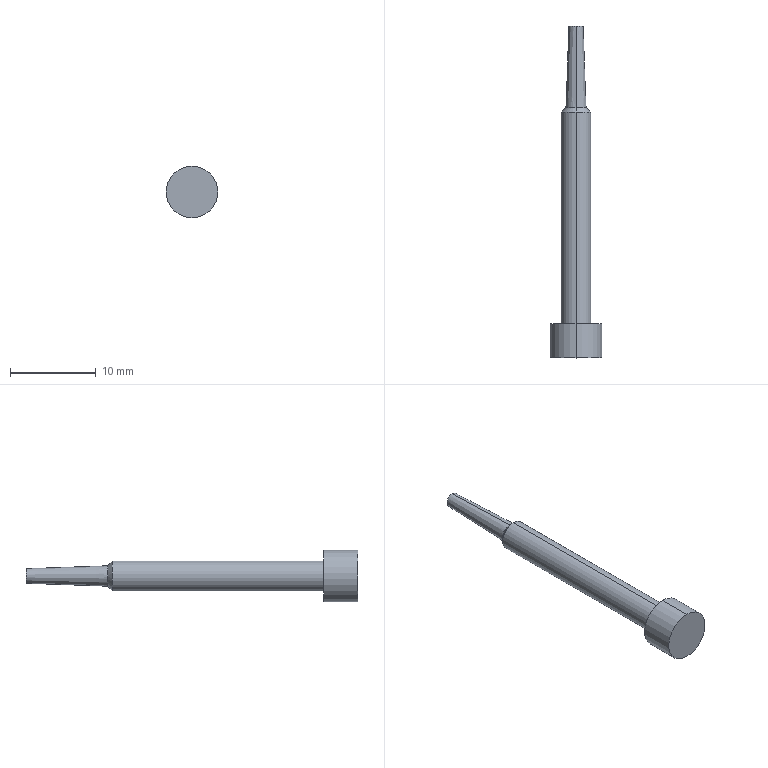Part | STEP file | 1 solid | 12 faces | box 6 x 38.743 x 6 mm | volume 385.655 mm3 | cylinder 4 | cone 4 | plane 4 | commonest cylinder face diameters 3.5 x2 6 x2
STEP:
#1=CARTESIAN_POINT('',(0.,0.,0.));
#2=DIRECTION('',(0.,0.,1.));
#3=DIRECTION('',(1.,0.,0.));
#4=AXIS2_PLACEMENT_3D('',#1,#2,#3);
#5=CARTESIAN_POINT('',(-137.183,-30.,14.557));
#6=VERTEX_POINT('',#5);
#7=CARTESIAN_POINT('',(-137.183,-30.,8.557));
#8=VERTEX_POINT('',#7);
#9=CARTESIAN_POINT('',(-137.183,-30.,11.557));
#10=DIRECTION('',(0.,1.,0.));
#11=DIRECTION('',(0.,0.,1.));
#12=AXIS2_PLACEMENT_3D('',#9,#10,#11);
#13=CIRCLE('',#12,3.);
#14=CARTESIAN_POINT('',(-137.183,-30.,11.557));
#15=DIRECTION('',(0.,1.,0.));
#16=DIRECTION('',(0.,0.,1.));
#17=AXIS2_PLACEMENT_3D('',#14,#15,#16);
#18=CYLINDRICAL_SURFACE('',#17,3.);
#19=CARTESIAN_POINT('',(0.,0.));
#20=DIRECTION('',(1.,0.));
#21=VECTOR('',#20,1.);
#22=LINE('',#19,#21);
#23=(GEOMETRIC_REPRESENTATION_CONTEXT(2)PARAMETRIC_REPRESENTATION_CONTEXT()REPRESENTATION_CONTEXT('',''));
#24=DEFINITIONAL_REPRESENTATION('',(#22),#23);
#25=PCURVE('',#18,#24);
#26=CARTESIAN_POINT('',(-72.862,-30.,115.03));
#27=DIRECTION('',(0.,1.,0.));
#28=DIRECTION('',(0.,0.,1.));
#29=AXIS2_PLACEMENT_3D('',#26,#27,#28);
#30=PLANE('',#29);
#31=CARTESIAN_POINT('',(-103.472,-64.32));
#32=DIRECTION('',(1.,0.));
#33=AXIS2_PLACEMENT_2D('',#31,#32);
#34=CIRCLE('',#33,3.);
#35=(GEOMETRIC_REPRESENTATION_CONTEXT(2)PARAMETRIC_REPRESENTATION_CONTEXT()REPRESENTATION_CONTEXT('',''));
#36=DEFINITIONAL_REPRESENTATION('',(#34),#35);
#37=PCURVE('',#30,#36);
#38=SURFACE_CURVE('',#13,(#25,#37),.PCURVE_S1.);
#39=EDGE_CURVE('',#6,#8,#38,.T.);
#40=ORIENTED_EDGE('',*,*,#39,.T.);
#41=CARTESIAN_POINT('',(-137.183,-26.,8.557));
#42=VERTEX_POINT('',#41);
#43=CARTESIAN_POINT('',(-137.183,-30.,8.557));
#44=DIRECTION('',(0.,1.,0.));
#45=VECTOR('',#44,1.);
#46=LINE('',#43,#45);
#47=CARTESIAN_POINT('',(3.142,0.));
#48=DIRECTION('',(0.,1.));
#49=VECTOR('',#48,1.);
#50=LINE('',#47,#49);
#51=(GEOMETRIC_REPRESENTATION_CONTEXT(2)PARAMETRIC_REPRESENTATION_CONTEXT()REPRESENTATION_CONTEXT('',''));
#52=DEFINITIONAL_REPRESENTATION('',(#50),#51);
#53=PCURVE('',#18,#52);
#54=CARTESIAN_POINT('',(-137.183,-30.,11.557));
#55=DIRECTION('',(0.,1.,0.));
#56=DIRECTION('',(0.,0.,1.));
#57=AXIS2_PLACEMENT_3D('',#54,#55,#56);
#58=CYLINDRICAL_SURFACE('',#57,3.);
#59=CARTESIAN_POINT('',(3.142,0.));
#60=DIRECTION('',(0.,1.));
#61=VECTOR('',#60,1.);
#62=LINE('',#59,#61);
#63=(GEOMETRIC_REPRESENTATION_CONTEXT(2)PARAMETRIC_REPRESENTATION_CONTEXT()REPRESENTATION_CONTEXT('',''));
#64=DEFINITIONAL_REPRESENTATION('',(#62),#63);
#65=PCURVE('',#58,#64);
#66=SURFACE_CURVE('',#46,(#53,#65),.PCURVE_S1.);
#67=EDGE_CURVE('',#8,#42,#66,.T.);
#68=ORIENTED_EDGE('',*,*,#67,.T.);
#69=CARTESIAN_POINT('',(-137.183,-26.,14.557));
#70=VERTEX_POINT('',#69);
#71=CARTESIAN_POINT('',(-137.183,-26.,11.557));
#72=DIRECTION('',(0.,-1.,0.));
#73=DIRECTION('',(0.,0.,-1.));
#74=AXIS2_PLACEMENT_3D('',#71,#72,#73);
#75=CIRCLE('',#74,3.);
#76=CARTESIAN_POINT('',(3.142,4.));
#77=DIRECTION('',(-1.,0.));
#78=VECTOR('',#77,1.);
#79=LINE('',#76,#78);
#80=(GEOMETRIC_REPRESENTATION_CONTEXT(2)PARAMETRIC_REPRESENTATION_CONTEXT()REPRESENTATION_CONTEXT('',''));
#81=DEFINITIONAL_REPRESENTATION('',(#79),#80);
#82=PCURVE('',#18,#81);
#83=CARTESIAN_POINT('',(-137.183,-26.,11.557));
#84=DIRECTION('',(0.,1.,0.));
#85=DIRECTION('',(0.,0.,1.));
#86=AXIS2_PLACEMENT_3D('',#83,#84,#85);
#87=PLANE('',#86);
#88=CARTESIAN_POINT('',(-3.,0.));
#89=CARTESIAN_POINT('',(-3.,5.196));
#90=CARTESIAN_POINT('',(1.5,2.598));
#91=CARTESIAN_POINT('',(6.,0.));
#92=CARTESIAN_POINT('',(1.5,-2.598));
#93=CARTESIAN_POINT('',(-3.,-5.196));
#94=CARTESIAN_POINT('',(-3.,0.));
#95=(BOUNDED_CURVE()B_SPLINE_CURVE(2,(#88,#89,#90,#91,#92,#93,#94),.UNSPECIFIED.,.T.,.F.)B_SPLINE_CURVE_WITH_KNOTS((1,2,2,2,2,1),(-2.094,0.,2.094,4.189,6.283,8.378),.UNSPECIFIED.)CURVE()GEOMETRIC_REPRESENTATION_ITEM()RATIONAL_B_SPLINE_CURVE((1.,0.5,1.,0.5,1.,0.5,1.))REPRESENTATION_ITEM(''));
#96=(GEOMETRIC_REPRESENTATION_CONTEXT(2)PARAMETRIC_REPRESENTATION_CONTEXT()REPRESENTATION_CONTEXT('',''));
#97=DEFINITIONAL_REPRESENTATION('',(#95),#96);
#98=PCURVE('',#87,#97);
#99=SURFACE_CURVE('',#75,(#82,#98),.PCURVE_S1.);
#100=EDGE_CURVE('',#42,#70,#99,.T.);
#101=ORIENTED_EDGE('',*,*,#100,.T.);
#102=CARTESIAN_POINT('',(-137.183,-30.,14.557));
#103=DIRECTION('',(0.,1.,0.));
#104=VECTOR('',#103,1.);
#105=LINE('',#102,#104);
#106=CARTESIAN_POINT('',(0.,0.));
#107=DIRECTION('',(0.,1.));
#108=VECTOR('',#107,1.);
#109=LINE('',#106,#108);
#110=(GEOMETRIC_REPRESENTATION_CONTEXT(2)PARAMETRIC_REPRESENTATION_CONTEXT()REPRESENTATION_CONTEXT('',''));
#111=DEFINITIONAL_REPRESENTATION('',(#109),#110);
#112=PCURVE('',#18,#111);
#113=CARTESIAN_POINT('',(6.283,0.));
#114=DIRECTION('',(0.,1.));
#115=VECTOR('',#114,1.);
#116=LINE('',#113,#115);
#117=(GEOMETRIC_REPRESENTATION_CONTEXT(2)PARAMETRIC_REPRESENTATION_CONTEXT()REPRESENTATION_CONTEXT('',''));
#118=DEFINITIONAL_REPRESENTATION('',(#116),#117);
#119=PCURVE('',#58,#118);
#120=SURFACE_CURVE('',#105,(#112,#119),.PCURVE_S1.);
#121=EDGE_CURVE('',#6,#70,#120,.T.);
#122=ORIENTED_EDGE('',*,*,#121,.F.);
#123=EDGE_LOOP('',(#40,#68,#101,#122));
#124=FACE_BOUND('',#123,.T.);
#125=ADVANCED_FACE('',(#124),#18,.T.);
#126=CARTESIAN_POINT('',(-137.183,-0.7858,10.37));
#127=VERTEX_POINT('',#126);
#128=CARTESIAN_POINT('',(-137.183,-0.7858,12.745));
#129=VERTEX_POINT('',#128);
#130=CARTESIAN_POINT('',(-137.183,-0.7858,11.557));
#131=DIRECTION('',(0.,-1.,0.));
#132=DIRECTION('',(0.,0.,1.));
#133=AXIS2_PLACEMENT_3D('',#130,#131,#132);
#134=CIRCLE('',#133,1.188);
#135=CARTESIAN_POINT('',(-137.183,-1.306,11.557));
#136=DIRECTION('',(0.,-1.,0.));
#137=DIRECTION('',(0.,0.,-1.));
#138=AXIS2_PLACEMENT_3D('',#135,#136,#137);
#139=CONICAL_SURFACE('',#138,1.708,0.7854);
#140=CARTESIAN_POINT('',(-3.142,-0.5207));
#141=DIRECTION('',(1.,0.));
#142=VECTOR('',#141,1.);
#143=LINE('',#140,#142);
#144=(GEOMETRIC_REPRESENTATION_CONTEXT(2)PARAMETRIC_REPRESENTATION_CONTEXT()REPRESENTATION_CONTEXT('',''));
#145=DEFINITIONAL_REPRESENTATION('',(#143),#144);
#146=PCURVE('',#139,#145);
#147=CARTESIAN_POINT('',(-137.183,-1.306,11.557));
#148=DIRECTION('',(0.,-1.,0.));
#149=DIRECTION('',(0.,0.,-1.));
#150=AXIS2_PLACEMENT_3D('',#147,#148,#149);
#151=CONICAL_SURFACE('',#150,1.206,0.03491);
#152=CARTESIAN_POINT('',(-3.142,-0.5207));
#153=DIRECTION('',(1.,0.));
#154=VECTOR('',#153,1.);
#155=LINE('',#152,#154);
#156=(GEOMETRIC_REPRESENTATION_CONTEXT(2)PARAMETRIC_REPRESENTATION_CONTEXT()REPRESENTATION_CONTEXT('',''));
#157=DEFINITIONAL_REPRESENTATION('',(#155),#156);
#158=PCURVE('',#151,#157);
#159=SURFACE_CURVE('',#134,(#146,#158),.PCURVE_S1.);
#160=EDGE_CURVE('',#127,#129,#159,.T.);
#161=ORIENTED_EDGE('',*,*,#160,.T.);
#162=CARTESIAN_POINT('',(-137.183,-1.306,13.266));
#163=VERTEX_POINT('',#162);
#164=CARTESIAN_POINT('',(-137.183,-1.306,13.266));
#165=DIRECTION('',(0.,-0.7071,0.7071));
#166=VECTOR('',#165,1.);
#167=LINE('',#164,#166);
#168=CARTESIAN_POINT('',(3.142,0.));
#169=DIRECTION('',(0.,1.));
#170=VECTOR('',#169,1.);
#171=LINE('',#168,#170);
#172=(GEOMETRIC_REPRESENTATION_CONTEXT(2)PARAMETRIC_REPRESENTATION_CONTEXT()REPRESENTATION_CONTEXT('',''));
#173=DEFINITIONAL_REPRESENTATION('',(#171),#172);
#174=PCURVE('',#139,#173);
#175=CARTESIAN_POINT('',(-137.183,-1.306,11.557));
#176=DIRECTION('',(0.,-1.,0.));
#177=DIRECTION('',(0.,0.,-1.));
#178=AXIS2_PLACEMENT_3D('',#175,#176,#177);
#179=CONICAL_SURFACE('',#178,1.708,0.7854);
#180=CARTESIAN_POINT('',(3.142,0.));
#181=DIRECTION('',(0.,1.));
#182=VECTOR('',#181,1.);
#183=LINE('',#180,#182);
#184=(GEOMETRIC_REPRESENTATION_CONTEXT(2)PARAMETRIC_REPRESENTATION_CONTEXT()REPRESENTATION_CONTEXT('',''));
#185=DEFINITIONAL_REPRESENTATION('',(#183),#184);
#186=PCURVE('',#179,#185);
#187=SURFACE_CURVE('',#167,(#174,#186),.PCURVE_S1.);
#188=EDGE_CURVE('',#129,#163,#187,.T.);
#189=ORIENTED_EDGE('',*,*,#188,.T.);
#190=CARTESIAN_POINT('',(-137.183,-1.306,9.849));
#191=VERTEX_POINT('',#190);
#192=CARTESIAN_POINT('',(-137.183,-1.306,11.557));
#193=DIRECTION('',(0.,1.,0.));
#194=DIRECTION('',(0.,0.,-1.));
#195=AXIS2_PLACEMENT_3D('',#192,#193,#194);
#196=CIRCLE('',#195,1.708);
#197=CARTESIAN_POINT('',(6.283,0.));
#198=DIRECTION('',(-1.,0.));
#199=VECTOR('',#198,1.);
#200=LINE('',#197,#199);
#201=(GEOMETRIC_REPRESENTATION_CONTEXT(2)PARAMETRIC_REPRESENTATION_CONTEXT()REPRESENTATION_CONTEXT('',''));
#202=DEFINITIONAL_REPRESENTATION('',(#200),#201);
#203=PCURVE('',#139,#202);
#204=CARTESIAN_POINT('',(-137.183,-1.306,11.557));
#205=DIRECTION('',(0.,1.,0.));
#206=DIRECTION('',(0.,0.,1.));
#207=AXIS2_PLACEMENT_3D('',#204,#205,#206);
#208=PLANE('',#207);
#209=CARTESIAN_POINT('',(0.,0.));
#210=DIRECTION('',(-1.,0.));
#211=AXIS2_PLACEMENT_2D('',#209,#210);
#212=CIRCLE('',#211,1.708);
#213=(GEOMETRIC_REPRESENTATION_CONTEXT(2)PARAMETRIC_REPRESENTATION_CONTEXT()REPRESENTATION_CONTEXT('',''));
#214=DEFINITIONAL_REPRESENTATION('',(#212),#213);
#215=PCURVE('',#208,#214);
#216=SURFACE_CURVE('',#196,(#203,#215),.PCURVE_S1.);
#217=EDGE_CURVE('',#163,#191,#216,.T.);
#218=ORIENTED_EDGE('',*,*,#217,.T.);
#219=CARTESIAN_POINT('',(-137.183,-1.306,9.849));
#220=DIRECTION('',(0.,-0.7071,-0.7071));
#221=VECTOR('',#220,1.);
#222=LINE('',#219,#221);
#223=CARTESIAN_POINT('',(0.,0.));
#224=DIRECTION('',(0.,1.));
#225=VECTOR('',#224,1.);
#226=LINE('',#223,#225);
#227=(GEOMETRIC_REPRESENTATION_CONTEXT(2)PARAMETRIC_REPRESENTATION_CONTEXT()REPRESENTATION_CONTEXT('',''));
#228=DEFINITIONAL_REPRESENTATION('',(#226),#227);
#229=PCURVE('',#139,#228);
#230=CARTESIAN_POINT('',(6.283,0.));
#231=DIRECTION('',(0.,1.));
#232=VECTOR('',#231,1.);
#233=LINE('',#230,#232);
#234=(GEOMETRIC_REPRESENTATION_CONTEXT(2)PARAMETRIC_REPRESENTATION_CONTEXT()REPRESENTATION_CONTEXT('',''));
#235=DEFINITIONAL_REPRESENTATION('',(#233),#234);
#236=PCURVE('',#179,#235);
#237=SURFACE_CURVE('',#222,(#229,#236),.PCURVE_S1.);
#238=EDGE_CURVE('',#127,#191,#237,.T.);
#239=ORIENTED_EDGE('',*,*,#238,.F.);
#240=EDGE_LOOP('',(#161,#189,#218,#239));
#241=FACE_BOUND('',#240,.T.);
#242=ADVANCED_FACE('',(#241),#139,.T.);
#243=CARTESIAN_POINT('',(-137.183,8.743,10.702));
#244=VERTEX_POINT('',#243);
#245=CARTESIAN_POINT('',(-137.183,8.743,12.413));
#246=VERTEX_POINT('',#245);
#247=CARTESIAN_POINT('',(-137.183,8.743,11.557));
#248=DIRECTION('',(0.,-1.,0.));
#249=DIRECTION('',(0.,0.,-1.));
#250=AXIS2_PLACEMENT_3D('',#247,#248,#249);
#251=CIRCLE('',#250,0.855);
#252=CARTESIAN_POINT('',(0.,-10.05));
#253=DIRECTION('',(1.,0.));
#254=VECTOR('',#253,1.);
#255=LINE('',#252,#254);
#256=(GEOMETRIC_REPRESENTATION_CONTEXT(2)PARAMETRIC_REPRESENTATION_CONTEXT()REPRESENTATION_CONTEXT('',''));
#257=DEFINITIONAL_REPRESENTATION('',(#255),#256);
#258=PCURVE('',#151,#257);
#259=CARTESIAN_POINT('',(-137.183,8.743,9.849));
#260=DIRECTION('',(0.,1.,0.));
#261=DIRECTION('',(0.,0.,1.));
#262=AXIS2_PLACEMENT_3D('',#259,#260,#261);
#263=PLANE('',#262);
#264=CARTESIAN_POINT('',(0.8535,0.));
#265=CARTESIAN_POINT('',(0.8535,1.481));
#266=CARTESIAN_POINT('',(2.136,0.7405));
#267=CARTESIAN_POINT('',(3.419,0.));
#268=CARTESIAN_POINT('',(2.136,-0.7405));
#269=CARTESIAN_POINT('',(0.8535,-1.481));
#270=CARTESIAN_POINT('',(0.8535,0.));
#271=(BOUNDED_CURVE()B_SPLINE_CURVE(2,(#264,#265,#266,#267,#268,#269,#270),.UNSPECIFIED.,.T.,.F.)B_SPLINE_CURVE_WITH_KNOTS((1,2,2,2,2,1),(-2.094,0.,2.094,4.189,6.283,8.378),.UNSPECIFIED.)CURVE()GEOMETRIC_REPRESENTATION_ITEM()RATIONAL_B_SPLINE_CURVE((1.,0.5,1.,0.5,1.,0.5,1.))REPRESENTATION_ITEM(''));
#272=(GEOMETRIC_REPRESENTATION_CONTEXT(2)PARAMETRIC_REPRESENTATION_CONTEXT()REPRESENTATION_CONTEXT('',''));
#273=DEFINITIONAL_REPRESENTATION('',(#271),#272);
#274=PCURVE('',#263,#273);
#275=SURFACE_CURVE('',#251,(#258,#274),.PCURVE_S1.);
#276=EDGE_CURVE('',#244,#246,#275,.T.);
#277=ORIENTED_EDGE('',*,*,#276,.T.);
#278=CARTESIAN_POINT('',(-137.183,-1.306,12.764));
#279=DIRECTION('',(0.,-0.9994,0.0349));
#280=VECTOR('',#279,1.);
#281=LINE('',#278,#280);
#282=CARTESIAN_POINT('',(3.142,0.));
#283=DIRECTION('',(0.,1.));
#284=VECTOR('',#283,1.);
#285=LINE('',#282,#284);
#286=(GEOMETRIC_REPRESENTATION_CONTEXT(2)PARAMETRIC_REPRESENTATION_CONTEXT()REPRESENTATION_CONTEXT('',''));
#287=DEFINITIONAL_REPRESENTATION('',(#285),#286);
#288=PCURVE('',#151,#287);
#289=CARTESIAN_POINT('',(-137.183,-1.306,11.557));
#290=DIRECTION('',(0.,-1.,0.));
#291=DIRECTION('',(0.,0.,-1.));
#292=AXIS2_PLACEMENT_3D('',#289,#290,#291);
#293=CONICAL_SURFACE('',#292,1.206,0.03491);
#294=CARTESIAN_POINT('',(3.142,0.));
#295=DIRECTION('',(0.,1.));
#296=VECTOR('',#295,1.);
#297=LINE('',#294,#296);
#298=(GEOMETRIC_REPRESENTATION_CONTEXT(2)PARAMETRIC_REPRESENTATION_CONTEXT()REPRESENTATION_CONTEXT('',''));
#299=DEFINITIONAL_REPRESENTATION('',(#297),#298);
#300=PCURVE('',#293,#299);
#301=SURFACE_CURVE('',#281,(#288,#300),.PCURVE_S1.);
#302=EDGE_CURVE('',#246,#129,#301,.T.);
#303=ORIENTED_EDGE('',*,*,#302,.T.);
#304=ORIENTED_EDGE('',*,*,#160,.F.);
#305=CARTESIAN_POINT('',(-137.183,-1.306,10.351));
#306=DIRECTION('',(0.,-0.9994,-0.0349));
#307=VECTOR('',#306,1.);
#308=LINE('',#305,#307);
#309=CARTESIAN_POINT('',(0.,0.));
#310=DIRECTION('',(0.,1.));
#311=VECTOR('',#310,1.);
#312=LINE('',#309,#311);
#313=(GEOMETRIC_REPRESENTATION_CONTEXT(2)PARAMETRIC_REPRESENTATION_CONTEXT()REPRESENTATION_CONTEXT('',''));
#314=DEFINITIONAL_REPRESENTATION('',(#312),#313);
#315=PCURVE('',#151,#314);
#316=CARTESIAN_POINT('',(6.283,0.));
#317=DIRECTION('',(0.,1.));
#318=VECTOR('',#317,1.);
#319=LINE('',#316,#318);
#320=(GEOMETRIC_REPRESENTATION_CONTEXT(2)PARAMETRIC_REPRESENTATION_CONTEXT()REPRESENTATION_CONTEXT('',''));
#321=DEFINITIONAL_REPRESENTATION('',(#319),#320);
#322=PCURVE('',#293,#321);
#323=SURFACE_CURVE('',#308,(#315,#322),.PCURVE_S1.);
#324=EDGE_CURVE('',#244,#127,#323,.T.);
#325=ORIENTED_EDGE('',*,*,#324,.F.);
#326=EDGE_LOOP('',(#277,#303,#304,#325));
#327=FACE_BOUND('',#326,.T.);
#328=ADVANCED_FACE('',(#327),#151,.T.);
#329=CARTESIAN_POINT('',(-137.183,-1.306,9.807));
#330=VERTEX_POINT('',#329);
#331=CARTESIAN_POINT('',(-137.183,-1.306,13.307));
#332=VERTEX_POINT('',#331);
#333=CARTESIAN_POINT('',(-137.183,-1.306,11.557));
#334=DIRECTION('',(0.,-1.,0.));
#335=DIRECTION('',(0.,0.,-1.));
#336=AXIS2_PLACEMENT_3D('',#333,#334,#335);
#337=CIRCLE('',#336,1.75);
#338=CARTESIAN_POINT('',(-137.183,-1.306,11.557));
#339=DIRECTION('',(0.,-1.,0.));
#340=DIRECTION('',(0.,0.,-1.));
#341=AXIS2_PLACEMENT_3D('',#338,#339,#340);
#342=CYLINDRICAL_SURFACE('',#341,1.75);
#343=CARTESIAN_POINT('',(0.,0.));
#344=DIRECTION('',(1.,0.));
#345=VECTOR('',#344,1.);
#346=LINE('',#343,#345);
#347=(GEOMETRIC_REPRESENTATION_CONTEXT(2)PARAMETRIC_REPRESENTATION_CONTEXT()REPRESENTATION_CONTEXT('',''));
#348=DEFINITIONAL_REPRESENTATION('',(#346),#347);
#349=PCURVE('',#342,#348);
#350=CARTESIAN_POINT('',(-1.75,0.));
#351=CARTESIAN_POINT('',(-1.75,3.031));
#352=CARTESIAN_POINT('',(0.875,1.516));
#353=CARTESIAN_POINT('',(3.5,0.));
#354=CARTESIAN_POINT('',(0.875,-1.516));
#355=CARTESIAN_POINT('',(-1.75,-3.031));
#356=CARTESIAN_POINT('',(-1.75,0.));
#357=(BOUNDED_CURVE()B_SPLINE_CURVE(2,(#350,#351,#352,#353,#354,#355,#356),.UNSPECIFIED.,.T.,.F.)B_SPLINE_CURVE_WITH_KNOTS((1,2,2,2,2,1),(-2.094,0.,2.094,4.189,6.283,8.378),.UNSPECIFIED.)CURVE()GEOMETRIC_REPRESENTATION_ITEM()RATIONAL_B_SPLINE_CURVE((1.,0.5,1.,0.5,1.,0.5,1.))REPRESENTATION_ITEM(''));
#358=(GEOMETRIC_REPRESENTATION_CONTEXT(2)PARAMETRIC_REPRESENTATION_CONTEXT()REPRESENTATION_CONTEXT('',''));
#359=DEFINITIONAL_REPRESENTATION('',(#357),#358);
#360=PCURVE('',#208,#359);
#361=SURFACE_CURVE('',#337,(#349,#360),.PCURVE_S1.);
#362=EDGE_CURVE('',#330,#332,#361,.T.);
#363=ORIENTED_EDGE('',*,*,#362,.T.);
#364=CARTESIAN_POINT('',(-137.183,-26.,13.307));
#365=VERTEX_POINT('',#364);
#366=CARTESIAN_POINT('',(-137.183,-1.306,13.307));
#367=DIRECTION('',(0.,-1.,0.));
#368=VECTOR('',#367,1.);
#369=LINE('',#366,#368);
#370=CARTESIAN_POINT('',(3.142,0.));
#371=DIRECTION('',(0.,1.));
#372=VECTOR('',#371,1.);
#373=LINE('',#370,#372);
#374=(GEOMETRIC_REPRESENTATION_CONTEXT(2)PARAMETRIC_REPRESENTATION_CONTEXT()REPRESENTATION_CONTEXT('',''));
#375=DEFINITIONAL_REPRESENTATION('',(#373),#374);
#376=PCURVE('',#342,#375);
#377=CARTESIAN_POINT('',(-137.183,-1.306,11.557));
#378=DIRECTION('',(0.,-1.,0.));
#379=DIRECTION('',(0.,0.,-1.));
#380=AXIS2_PLACEMENT_3D('',#377,#378,#379);
#381=CYLINDRICAL_SURFACE('',#380,1.75);
#382=CARTESIAN_POINT('',(3.142,0.));
#383=DIRECTION('',(0.,1.));
#384=VECTOR('',#383,1.);
#385=LINE('',#382,#384);
#386=(GEOMETRIC_REPRESENTATION_CONTEXT(2)PARAMETRIC_REPRESENTATION_CONTEXT()REPRESENTATION_CONTEXT('',''));
#387=DEFINITIONAL_REPRESENTATION('',(#385),#386);
#388=PCURVE('',#381,#387);
#389=SURFACE_CURVE('',#369,(#376,#388),.PCURVE_S1.);
#390=EDGE_CURVE('',#332,#365,#389,.T.);
#391=ORIENTED_EDGE('',*,*,#390,.T.);
#392=CARTESIAN_POINT('',(-137.183,-26.,9.807));
#393=VERTEX_POINT('',#392);
#394=CARTESIAN_POINT('',(-137.183,-26.,11.557));
#395=DIRECTION('',(0.,-1.,0.));
#396=DIRECTION('',(0.,0.,1.));
#397=AXIS2_PLACEMENT_3D('',#394,#395,#396);
#398=CIRCLE('',#397,1.75);
#399=CARTESIAN_POINT('',(-3.142,24.694));
#400=DIRECTION('',(1.,0.));
#401=VECTOR('',#400,1.);
#402=LINE('',#399,#401);
#403=(GEOMETRIC_REPRESENTATION_CONTEXT(2)PARAMETRIC_REPRESENTATION_CONTEXT()REPRESENTATION_CONTEXT('',''));
#404=DEFINITIONAL_REPRESENTATION('',(#402),#403);
#405=PCURVE('',#342,#404);
#406=CARTESIAN_POINT('',(1.75,0.));
#407=CARTESIAN_POINT('',(1.75,-3.031));
#408=CARTESIAN_POINT('',(-0.875,-1.516));
#409=CARTESIAN_POINT('',(-3.5,0.));
#410=CARTESIAN_POINT('',(-0.875,1.516));
#411=CARTESIAN_POINT('',(1.75,3.031));
#412=CARTESIAN_POINT('',(1.75,0.));
#413=(BOUNDED_CURVE()B_SPLINE_CURVE(2,(#406,#407,#408,#409,#410,#411,#412),.UNSPECIFIED.,.T.,.F.)B_SPLINE_CURVE_WITH_KNOTS((1,2,2,2,2,1),(-2.094,0.,2.094,4.189,6.283,8.378),.UNSPECIFIED.)CURVE()GEOMETRIC_REPRESENTATION_ITEM()RATIONAL_B_SPLINE_CURVE((1.,0.5,1.,0.5,1.,0.5,1.))REPRESENTATION_ITEM(''));
#414=(GEOMETRIC_REPRESENTATION_CONTEXT(2)PARAMETRIC_REPRESENTATION_CONTEXT()REPRESENTATION_CONTEXT('',''));
#415=DEFINITIONAL_REPRESENTATION('',(#413),#414);
#416=PCURVE('',#87,#415);
#417=SURFACE_CURVE('',#398,(#405,#416),.PCURVE_S1.);
#418=EDGE_CURVE('',#393,#365,#417,.T.);
#419=ORIENTED_EDGE('',*,*,#418,.F.);
#420=CARTESIAN_POINT('',(-137.183,-1.306,9.807));
#421=DIRECTION('',(0.,-1.,0.));
#422=VECTOR('',#421,1.);
#423=LINE('',#420,#422);
#424=CARTESIAN_POINT('',(0.,0.));
#425=DIRECTION('',(0.,1.));
#426=VECTOR('',#425,1.);
#427=LINE('',#424,#426);
#428=(GEOMETRIC_REPRESENTATION_CONTEXT(2)PARAMETRIC_REPRESENTATION_CONTEXT()REPRESENTATION_CONTEXT('',''));
#429=DEFINITIONAL_REPRESENTATION('',(#427),#428);
#430=PCURVE('',#342,#429);
#431=CARTESIAN_POINT('',(6.283,0.));
#432=DIRECTION('',(0.,1.));
#433=VECTOR('',#432,1.);
#434=LINE('',#431,#433);
#435=(GEOMETRIC_REPRESENTATION_CONTEXT(2)PARAMETRIC_REPRESENTATION_CONTEXT()REPRESENTATION_CONTEXT('',''));
#436=DEFINITIONAL_REPRESENTATION('',(#434),#435);
#437=PCURVE('',#381,#436);
#438=SURFACE_CURVE('',#423,(#430,#437),.PCURVE_S1.);
#439=EDGE_CURVE('',#330,#393,#438,.T.);
#440=ORIENTED_EDGE('',*,*,#439,.F.);
#441=EDGE_LOOP('',(#363,#391,#419,#440));
#442=FACE_BOUND('',#441,.T.);
#443=ADVANCED_FACE('',(#442),#342,.T.);
#444=CARTESIAN_POINT('',(-137.183,-1.306,11.557));
#445=DIRECTION('',(0.,1.,0.));
#446=DIRECTION('',(0.,0.,-1.));
#447=AXIS2_PLACEMENT_3D('',#444,#445,#446);
#448=CIRCLE('',#447,1.708);
#449=CARTESIAN_POINT('',(0.,0.));
#450=DIRECTION('',(-1.,0.));
#451=AXIS2_PLACEMENT_2D('',#449,#450);
#452=CIRCLE('',#451,1.708);
#453=(GEOMETRIC_REPRESENTATION_CONTEXT(2)PARAMETRIC_REPRESENTATION_CONTEXT()REPRESENTATION_CONTEXT('',''));
#454=DEFINITIONAL_REPRESENTATION('',(#452),#453);
#455=PCURVE('',#208,#454);
#456=CARTESIAN_POINT('',(6.283,0.));
#457=DIRECTION('',(-1.,0.));
#458=VECTOR('',#457,1.);
#459=LINE('',#456,#458);
#460=(GEOMETRIC_REPRESENTATION_CONTEXT(2)PARAMETRIC_REPRESENTATION_CONTEXT()REPRESENTATION_CONTEXT('',''));
#461=DEFINITIONAL_REPRESENTATION('',(#459),#460);
#462=PCURVE('',#179,#461);
#463=SURFACE_CURVE('',#448,(#455,#462),.PCURVE_S1.);
#464=EDGE_CURVE('',#191,#163,#463,.T.);
#465=ORIENTED_EDGE('',*,*,#464,.F.);
#466=ORIENTED_EDGE('',*,*,#217,.F.);
#467=EDGE_LOOP('',(#465,#466));
#468=FACE_BOUND('',#467,.T.);
#469=ORIENTED_EDGE('',*,*,#362,.F.);
#470=CARTESIAN_POINT('',(-137.183,-1.306,11.557));
#471=DIRECTION('',(0.,-1.,0.));
#472=DIRECTION('',(0.,0.,-1.));
#473=AXIS2_PLACEMENT_3D('',#470,#471,#472);
#474=CIRCLE('',#473,1.75);
#475=CARTESIAN_POINT('',(-1.75,0.));
#476=CARTESIAN_POINT('',(-1.75,3.031));
#477=CARTESIAN_POINT('',(0.875,1.516));
#478=CARTESIAN_POINT('',(3.5,0.));
#479=CARTESIAN_POINT('',(0.875,-1.516));
#480=CARTESIAN_POINT('',(-1.75,-3.031));
#481=CARTESIAN_POINT('',(-1.75,0.));
#482=(BOUNDED_CURVE()B_SPLINE_CURVE(2,(#475,#476,#477,#478,#479,#480,#481),.UNSPECIFIED.,.T.,.F.)B_SPLINE_CURVE_WITH_KNOTS((1,2,2,2,2,1),(-2.094,0.,2.094,4.189,6.283,8.378),.UNSPECIFIED.)CURVE()GEOMETRIC_REPRESENTATION_ITEM()RATIONAL_B_SPLINE_CURVE((1.,0.5,1.,0.5,1.,0.5,1.))REPRESENTATION_ITEM(''));
#483=(GEOMETRIC_REPRESENTATION_CONTEXT(2)PARAMETRIC_REPRESENTATION_CONTEXT()REPRESENTATION_CONTEXT('',''));
#484=DEFINITIONAL_REPRESENTATION('',(#482),#483);
#485=PCURVE('',#208,#484);
#486=CARTESIAN_POINT('',(0.,0.));
#487=DIRECTION('',(1.,0.));
#488=VECTOR('',#487,1.);
#489=LINE('',#486,#488);
#490=(GEOMETRIC_REPRESENTATION_CONTEXT(2)PARAMETRIC_REPRESENTATION_CONTEXT()REPRESENTATION_CONTEXT('',''));
#491=DEFINITIONAL_REPRESENTATION('',(#489),#490);
#492=PCURVE('',#381,#491);
#493=SURFACE_CURVE('',#474,(#485,#492),.PCURVE_S1.);
#494=EDGE_CURVE('',#332,#330,#493,.T.);
#495=ORIENTED_EDGE('',*,*,#494,.F.);
#496=EDGE_LOOP('',(#469,#495));
#497=FACE_BOUND('',#496,.T.);
#498=ADVANCED_FACE('',(#468,#497),#208,.T.);
#499=ORIENTED_EDGE('',*,*,#390,.F.);
#500=ORIENTED_EDGE('',*,*,#494,.T.);
#501=ORIENTED_EDGE('',*,*,#439,.T.);
#502=CARTESIAN_POINT('',(-137.183,-26.,11.557));
#503=DIRECTION('',(0.,-1.,0.));
#504=DIRECTION('',(0.,0.,1.));
#505=AXIS2_PLACEMENT_3D('',#502,#503,#504);
#506=CIRCLE('',#505,1.75);
#507=CARTESIAN_POINT('',(3.142,24.694));
#508=DIRECTION('',(1.,0.));
#509=VECTOR('',#508,1.);
#510=LINE('',#507,#509);
#511=(GEOMETRIC_REPRESENTATION_CONTEXT(2)PARAMETRIC_REPRESENTATION_CONTEXT()REPRESENTATION_CONTEXT('',''));
#512=DEFINITIONAL_REPRESENTATION('',(#510),#511);
#513=PCURVE('',#381,#512);
#514=CARTESIAN_POINT('',(1.75,0.));
#515=CARTESIAN_POINT('',(1.75,-3.031));
#516=CARTESIAN_POINT('',(-0.875,-1.516));
#517=CARTESIAN_POINT('',(-3.5,0.));
#518=CARTESIAN_POINT('',(-0.875,1.516));
#519=CARTESIAN_POINT('',(1.75,3.031));
#520=CARTESIAN_POINT('',(1.75,0.));
#521=(BOUNDED_CURVE()B_SPLINE_CURVE(2,(#514,#515,#516,#517,#518,#519,#520),.UNSPECIFIED.,.T.,.F.)B_SPLINE_CURVE_WITH_KNOTS((1,2,2,2,2,1),(-2.094,0.,2.094,4.189,6.283,8.378),.UNSPECIFIED.)CURVE()GEOMETRIC_REPRESENTATION_ITEM()RATIONAL_B_SPLINE_CURVE((1.,0.5,1.,0.5,1.,0.5,1.))REPRESENTATION_ITEM(''));
#522=(GEOMETRIC_REPRESENTATION_CONTEXT(2)PARAMETRIC_REPRESENTATION_CONTEXT()REPRESENTATION_CONTEXT('',''));
#523=DEFINITIONAL_REPRESENTATION('',(#521),#522);
#524=PCURVE('',#87,#523);
#525=SURFACE_CURVE('',#506,(#513,#524),.PCURVE_S1.);
#526=EDGE_CURVE('',#365,#393,#525,.T.);
#527=ORIENTED_EDGE('',*,*,#526,.F.);
#528=EDGE_LOOP('',(#499,#500,#501,#527));
#529=FACE_BOUND('',#528,.T.);
#530=ADVANCED_FACE('',(#529),#381,.T.);
#531=ORIENTED_EDGE('',*,*,#302,.F.);
#532=CARTESIAN_POINT('',(-137.183,8.743,11.557));
#533=DIRECTION('',(0.,-1.,0.));
#534=DIRECTION('',(0.,0.,-1.));
#535=AXIS2_PLACEMENT_3D('',#532,#533,#534);
#536=CIRCLE('',#535,0.855);
#537=CARTESIAN_POINT('',(0.,-10.05));
#538=DIRECTION('',(1.,0.));
#539=VECTOR('',#538,1.);
#540=LINE('',#537,#539);
#541=(GEOMETRIC_REPRESENTATION_CONTEXT(2)PARAMETRIC_REPRESENTATION_CONTEXT()REPRESENTATION_CONTEXT('',''));
#542=DEFINITIONAL_REPRESENTATION('',(#540),#541);
#543=PCURVE('',#293,#542);
#544=CARTESIAN_POINT('',(0.8535,0.));
#545=CARTESIAN_POINT('',(0.8535,1.481));
#546=CARTESIAN_POINT('',(2.136,0.7405));
#547=CARTESIAN_POINT('',(3.419,0.));
#548=CARTESIAN_POINT('',(2.136,-0.7405));
#549=CARTESIAN_POINT('',(0.8535,-1.481));
#550=CARTESIAN_POINT('',(0.8535,0.));
#551=(BOUNDED_CURVE()B_SPLINE_CURVE(2,(#544,#545,#546,#547,#548,#549,#550),.UNSPECIFIED.,.T.,.F.)B_SPLINE_CURVE_WITH_KNOTS((1,2,2,2,2,1),(-2.094,0.,2.094,4.189,6.283,8.378),.UNSPECIFIED.)CURVE()GEOMETRIC_REPRESENTATION_ITEM()RATIONAL_B_SPLINE_CURVE((1.,0.5,1.,0.5,1.,0.5,1.))REPRESENTATION_ITEM(''));
#552=(GEOMETRIC_REPRESENTATION_CONTEXT(2)PARAMETRIC_REPRESENTATION_CONTEXT()REPRESENTATION_CONTEXT('',''));
#553=DEFINITIONAL_REPRESENTATION('',(#551),#552);
#554=PCURVE('',#263,#553);
#555=SURFACE_CURVE('',#536,(#543,#554),.PCURVE_S1.);
#556=EDGE_CURVE('',#246,#244,#555,.T.);
#557=ORIENTED_EDGE('',*,*,#556,.T.);
#558=ORIENTED_EDGE('',*,*,#324,.T.);
#559=CARTESIAN_POINT('',(-137.183,-0.7858,11.557));
#560=DIRECTION('',(0.,-1.,0.));
#561=DIRECTION('',(0.,0.,1.));
#562=AXIS2_PLACEMENT_3D('',#559,#560,#561);
#563=CIRCLE('',#562,1.188);
#564=CARTESIAN_POINT('',(3.142,-0.5207));
#565=DIRECTION('',(1.,0.));
#566=VECTOR('',#565,1.);
#567=LINE('',#564,#566);
#568=(GEOMETRIC_REPRESENTATION_CONTEXT(2)PARAMETRIC_REPRESENTATION_CONTEXT()REPRESENTATION_CONTEXT('',''));
#569=DEFINITIONAL_REPRESENTATION('',(#567),#568);
#570=PCURVE('',#293,#569);
#571=CARTESIAN_POINT('',(3.142,-0.5207));
#572=DIRECTION('',(1.,0.));
#573=VECTOR('',#572,1.);
#574=LINE('',#571,#573);
#575=(GEOMETRIC_REPRESENTATION_CONTEXT(2)PARAMETRIC_REPRESENTATION_CONTEXT()REPRESENTATION_CONTEXT('',''));
#576=DEFINITIONAL_REPRESENTATION('',(#574),#575);
#577=PCURVE('',#179,#576);
#578=SURFACE_CURVE('',#563,(#570,#577),.PCURVE_S1.);
#579=EDGE_CURVE('',#129,#127,#578,.T.);
#580=ORIENTED_EDGE('',*,*,#579,.F.);
#581=EDGE_LOOP('',(#531,#557,#558,#580));
#582=FACE_BOUND('',#581,.T.);
#583=ADVANCED_FACE('',(#582),#293,.T.);
#584=ORIENTED_EDGE('',*,*,#188,.F.);
#585=ORIENTED_EDGE('',*,*,#579,.T.);
#586=ORIENTED_EDGE('',*,*,#238,.T.);
#587=ORIENTED_EDGE('',*,*,#464,.T.);
#588=EDGE_LOOP('',(#584,#585,#586,#587));
#589=FACE_BOUND('',#588,.T.);
#590=ADVANCED_FACE('',(#589),#179,.T.);
#591=ORIENTED_EDGE('',*,*,#276,.F.);
#592=ORIENTED_EDGE('',*,*,#556,.F.);
#593=EDGE_LOOP('',(#591,#592));
#594=FACE_BOUND('',#593,.T.);
#595=ADVANCED_FACE('',(#594),#263,.T.);
#596=ORIENTED_EDGE('',*,*,#418,.T.);
#597=ORIENTED_EDGE('',*,*,#526,.T.);
#598=EDGE_LOOP('',(#596,#597));
#599=FACE_BOUND('',#598,.T.);
#600=CARTESIAN_POINT('',(-137.183,-26.,11.557));
#601=DIRECTION('',(0.,-1.,0.));
#602=DIRECTION('',(0.,0.,-1.));
#603=AXIS2_PLACEMENT_3D('',#600,#601,#602);
#604=CIRCLE('',#603,3.);
#605=CARTESIAN_POINT('',(-3.,0.));
#606=CARTESIAN_POINT('',(-3.,5.196));
#607=CARTESIAN_POINT('',(1.5,2.598));
#608=CARTESIAN_POINT('',(6.,0.));
#609=CARTESIAN_POINT('',(1.5,-2.598));
#610=CARTESIAN_POINT('',(-3.,-5.196));
#611=CARTESIAN_POINT('',(-3.,0.));
#612=(BOUNDED_CURVE()B_SPLINE_CURVE(2,(#605,#606,#607,#608,#609,#610,#611),.UNSPECIFIED.,.T.,.F.)B_SPLINE_CURVE_WITH_KNOTS((1,2,2,2,2,1),(-2.094,0.,2.094,4.189,6.283,8.378),.UNSPECIFIED.)CURVE()GEOMETRIC_REPRESENTATION_ITEM()RATIONAL_B_SPLINE_CURVE((1.,0.5,1.,0.5,1.,0.5,1.))REPRESENTATION_ITEM(''));
#613=(GEOMETRIC_REPRESENTATION_CONTEXT(2)PARAMETRIC_REPRESENTATION_CONTEXT()REPRESENTATION_CONTEXT('',''));
#614=DEFINITIONAL_REPRESENTATION('',(#612),#613);
#615=PCURVE('',#87,#614);
#616=CARTESIAN_POINT('',(9.425,4.));
#617=DIRECTION('',(-1.,0.));
#618=VECTOR('',#617,1.);
#619=LINE('',#616,#618);
#620=(GEOMETRIC_REPRESENTATION_CONTEXT(2)PARAMETRIC_REPRESENTATION_CONTEXT()REPRESENTATION_CONTEXT('',''));
#621=DEFINITIONAL_REPRESENTATION('',(#619),#620);
#622=PCURVE('',#58,#621);
#623=SURFACE_CURVE('',#604,(#615,#622),.PCURVE_S1.);
#624=EDGE_CURVE('',#70,#42,#623,.T.);
#625=ORIENTED_EDGE('',*,*,#624,.F.);
#626=ORIENTED_EDGE('',*,*,#100,.F.);
#627=EDGE_LOOP('',(#625,#626));
#628=FACE_BOUND('',#627,.T.);
#629=ADVANCED_FACE('',(#599,#628),#87,.T.);
#630=ORIENTED_EDGE('',*,*,#67,.F.);
#631=CARTESIAN_POINT('',(-137.183,-30.,11.557));
#632=DIRECTION('',(0.,1.,0.));
#633=DIRECTION('',(0.,0.,1.));
#634=AXIS2_PLACEMENT_3D('',#631,#632,#633);
#635=CIRCLE('',#634,3.);
#636=CARTESIAN_POINT('',(0.,0.));
#637=DIRECTION('',(1.,0.));
#638=VECTOR('',#637,1.);
#639=LINE('',#636,#638);
#640=(GEOMETRIC_REPRESENTATION_CONTEXT(2)PARAMETRIC_REPRESENTATION_CONTEXT()REPRESENTATION_CONTEXT('',''));
#641=DEFINITIONAL_REPRESENTATION('',(#639),#640);
#642=PCURVE('',#58,#641);
#643=CARTESIAN_POINT('',(-103.472,-64.32));
#644=DIRECTION('',(1.,0.));
#645=AXIS2_PLACEMENT_2D('',#643,#644);
#646=CIRCLE('',#645,3.);
#647=(GEOMETRIC_REPRESENTATION_CONTEXT(2)PARAMETRIC_REPRESENTATION_CONTEXT()REPRESENTATION_CONTEXT('',''));
#648=DEFINITIONAL_REPRESENTATION('',(#646),#647);
#649=PCURVE('',#30,#648);
#650=SURFACE_CURVE('',#635,(#642,#649),.PCURVE_S1.);
#651=EDGE_CURVE('',#8,#6,#650,.T.);
#652=ORIENTED_EDGE('',*,*,#651,.T.);
#653=ORIENTED_EDGE('',*,*,#121,.T.);
#654=ORIENTED_EDGE('',*,*,#624,.T.);
#655=EDGE_LOOP('',(#630,#652,#653,#654));
#656=FACE_BOUND('',#655,.T.);
#657=ADVANCED_FACE('',(#656),#58,.T.);
#658=ORIENTED_EDGE('',*,*,#39,.F.);
#659=ORIENTED_EDGE('',*,*,#651,.F.);
#660=EDGE_LOOP('',(#658,#659));
#661=FACE_BOUND('',#660,.T.);
#662=ADVANCED_FACE('',(#661),#30,.F.);
#663=CLOSED_SHELL('',(#125,#242,#328,#443,#498,#530,#583,#590,#595,#629,#657,#662));
#664=MANIFOLD_SOLID_BREP('',#663);
#665=(LENGTH_UNIT()NAMED_UNIT(*)SI_UNIT(.MILLI.,.METRE.));
#666=UNCERTAINTY_MEASURE_WITH_UNIT(LENGTH_MEASURE(0.0000001),#665,'','');
#667=(NAMED_UNIT(*)PLANE_ANGLE_UNIT()SI_UNIT($,.RADIAN.));
#668=(NAMED_UNIT(*)SI_UNIT($,.STERADIAN.)SOLID_ANGLE_UNIT());
#669=(GEOMETRIC_REPRESENTATION_CONTEXT(3)GLOBAL_UNCERTAINTY_ASSIGNED_CONTEXT((#666))GLOBAL_UNIT_ASSIGNED_CONTEXT((#665,#667,#668))REPRESENTATION_CONTEXT('',''));
#670=ADVANCED_BREP_SHAPE_REPRESENTATION('',(#4,#664),#669);